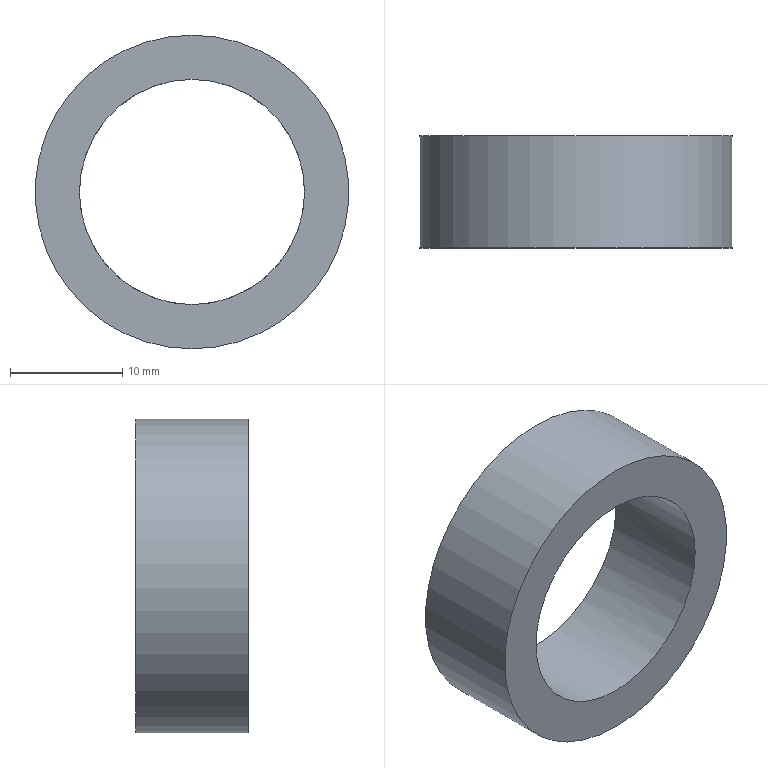Part | STEP file | 冲床-300配套压波_id1078_x_t | 1 solid | 4 faces | box 28 x 10 x 28 mm | volume 2984 mm3 | plane 2 | cylinder 2 | commonest cylinder face diameters 20.1 x1 28 x1
STEP:
#1=CARTESIAN_POINT('',(1250.,65.5,162.3));
#2=VERTEX_POINT('',#1);
#3=CARTESIAN_POINT('',(1250.,65.5,172.35));
#4=DIRECTION('',(0.,-1.,0.));
#5=DIRECTION('',(0.,0.,-1.));
#6=AXIS2_PLACEMENT_3D('',#3,#4,#5);
#7=CIRCLE('',#6,10.05);
#8=EDGE_CURVE('',#2,#2,#7,.T.);
#9=ORIENTED_EDGE('',*,*,#8,.F.);
#10=EDGE_LOOP('',(#9));
#11=FACE_BOUND('',#10,.T.);
#12=CARTESIAN_POINT('',(1250.,65.5,158.35));
#13=VERTEX_POINT('',#12);
#14=CARTESIAN_POINT('',(1250.,65.5,172.35));
#15=DIRECTION('',(0.,-1.,0.));
#16=DIRECTION('',(0.,0.,-1.));
#17=AXIS2_PLACEMENT_3D('',#14,#15,#16);
#18=CIRCLE('',#17,14.);
#19=EDGE_CURVE('',#13,#13,#18,.T.);
#20=ORIENTED_EDGE('',*,*,#19,.T.);
#21=EDGE_LOOP('',(#20));
#22=FACE_BOUND('',#21,.T.);
#23=CARTESIAN_POINT('',(1215.374,65.5,171.661));
#24=DIRECTION('',(0.,-1.,0.));
#25=DIRECTION('',(1.,0.,0.));
#26=AXIS2_PLACEMENT_3D('',#23,#24,#25);
#27=PLANE('',#26);
#28=ADVANCED_FACE('',(#11,#22),#27,.T.);
#29=CARTESIAN_POINT('',(1250.,75.5,186.35));
#30=VERTEX_POINT('',#29);
#31=CARTESIAN_POINT('',(1250.,75.5,172.35));
#32=DIRECTION('',(0.,-1.,0.));
#33=DIRECTION('',(0.,0.,1.));
#34=AXIS2_PLACEMENT_3D('',#31,#32,#33);
#35=CIRCLE('',#34,14.);
#36=EDGE_CURVE('',#30,#30,#35,.T.);
#37=ORIENTED_EDGE('',*,*,#36,.T.);
#38=EDGE_LOOP('',(#37));
#39=FACE_BOUND('',#38,.T.);
#40=ORIENTED_EDGE('',*,*,#19,.F.);
#41=EDGE_LOOP('',(#40));
#42=FACE_BOUND('',#41,.T.);
#43=CARTESIAN_POINT('',(1250.,-42.3,172.35));
#44=DIRECTION('',(0.,1.,0.));
#45=DIRECTION('',(0.,0.,1.));
#46=AXIS2_PLACEMENT_3D('',#43,#44,#45);
#47=CYLINDRICAL_SURFACE('',#46,14.);
#48=ADVANCED_FACE('',(#39,#42),#47,.T.);
#49=CARTESIAN_POINT('',(1250.,75.5,182.4));
#50=VERTEX_POINT('',#49);
#51=CARTESIAN_POINT('',(1250.,75.5,172.35));
#52=DIRECTION('',(0.,-1.,0.));
#53=DIRECTION('',(0.,0.,1.));
#54=AXIS2_PLACEMENT_3D('',#51,#52,#53);
#55=CIRCLE('',#54,10.05);
#56=EDGE_CURVE('',#50,#50,#55,.T.);
#57=ORIENTED_EDGE('',*,*,#56,.F.);
#58=EDGE_LOOP('',(#57));
#59=FACE_BOUND('',#58,.T.);
#60=ORIENTED_EDGE('',*,*,#8,.T.);
#61=EDGE_LOOP('',(#60));
#62=FACE_BOUND('',#61,.T.);
#63=CARTESIAN_POINT('',(1250.,-42.3,172.35));
#64=DIRECTION('',(0.,1.,0.));
#65=DIRECTION('',(0.,0.,1.));
#66=AXIS2_PLACEMENT_3D('',#63,#64,#65);
#67=CYLINDRICAL_SURFACE('',#66,10.05);
#68=ADVANCED_FACE('',(#59,#62),#67,.F.);
#69=ORIENTED_EDGE('',*,*,#36,.F.);
#70=EDGE_LOOP('',(#69));
#71=FACE_BOUND('',#70,.T.);
#72=ORIENTED_EDGE('',*,*,#56,.T.);
#73=EDGE_LOOP('',(#72));
#74=FACE_BOUND('',#73,.T.);
#75=CARTESIAN_POINT('',(1250.,75.5,172.35));
#76=DIRECTION('',(0.,1.,0.));
#77=DIRECTION('',(0.,0.,1.));
#78=AXIS2_PLACEMENT_3D('',#75,#76,#77);
#79=PLANE('',#78);
#80=ADVANCED_FACE('',(#71,#74),#79,.T.);
#81=CLOSED_SHELL('',(#28,#48,#68,#80));
#82=MANIFOLD_SOLID_BREP('',#81);
#83=(LENGTH_UNIT()NAMED_UNIT(*)SI_UNIT(.MILLI.,.METRE.));
#84=UNCERTAINTY_MEASURE_WITH_UNIT(LENGTH_MEASURE(0.00002),#83,'','');
#85=(NAMED_UNIT(*)PLANE_ANGLE_UNIT()SI_UNIT($,.RADIAN.));
#86=PLANE_ANGLE_MEASURE_WITH_UNIT(PLANE_ANGLE_MEASURE(0.01745),#85);
#87=DIMENSIONAL_EXPONENTS(0.,0.,0.,0.,0.,0.,0.);
#88=(CONVERSION_BASED_UNIT('DEGREE',#86)NAMED_UNIT(#87)PLANE_ANGLE_UNIT());
#89=(NAMED_UNIT(*)SI_UNIT($,.STERADIAN.)SOLID_ANGLE_UNIT());
#90=(GEOMETRIC_REPRESENTATION_CONTEXT(3)GLOBAL_UNCERTAINTY_ASSIGNED_CONTEXT((#84))GLOBAL_UNIT_ASSIGNED_CONTEXT((#83,#88,#89))REPRESENTATION_CONTEXT('',''));
#91=ADVANCED_BREP_SHAPE_REPRESENTATION('',(#82),#90);